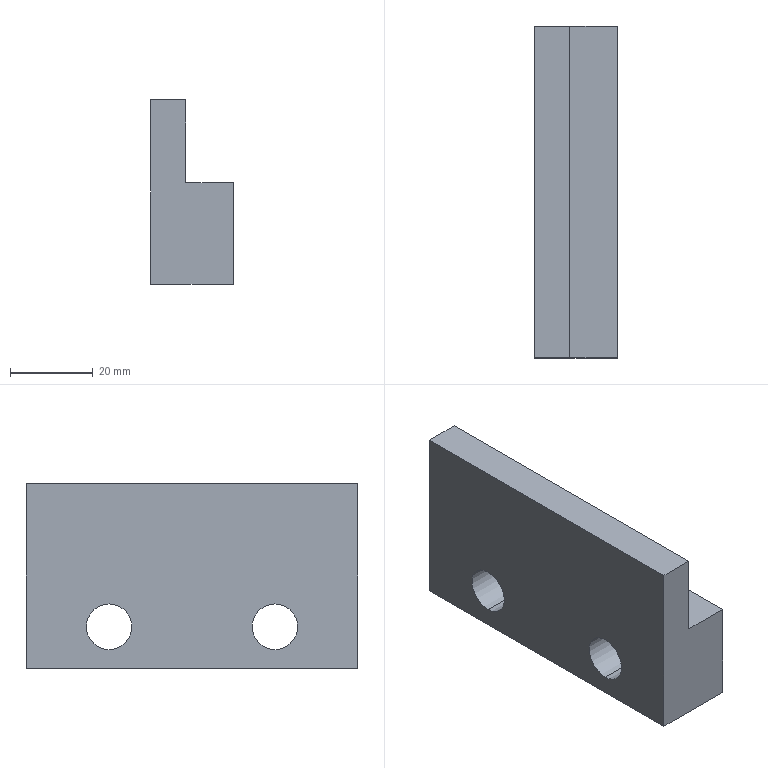Part | SolidWorks | features Extrusion 1, ICE 1 | 1 solid | 12 faces | box 20 x 80 x 44.5 mm | volume 48999 mm3 | plane 8 | cylinder 4 | commonest cylinder face diameters 11 x4
STEP:
#1=CARTESIAN_POINT('',(20.,-20.,-6.75));
#2=VERTEX_POINT('',#1);
#3=CARTESIAN_POINT('',(20.,-20.,-17.75));
#4=VERTEX_POINT('',#3);
#5=CARTESIAN_POINT('',(20.,-20.,-12.25));
#6=DIRECTION('',(1.,0.,0.));
#7=DIRECTION('',(0.,0.,-1.));
#8=AXIS2_PLACEMENT_3D('',#5,#6,#7);
#9=CIRCLE('',#8,5.5);
#10=EDGE_CURVE('',#2,#4,#9,.T.);
#11=ORIENTED_EDGE('',*,*,#10,.T.);
#12=CARTESIAN_POINT('',(0.,-20.,-17.75));
#13=VERTEX_POINT('',#12);
#14=CARTESIAN_POINT('',(20.,-20.,-17.75));
#15=DIRECTION('',(-1.,0.,0.));
#16=VECTOR('',#15,1000.);
#17=LINE('',#14,#16);
#18=EDGE_CURVE('',#4,#13,#17,.T.);
#19=ORIENTED_EDGE('',*,*,#18,.T.);
#20=CARTESIAN_POINT('',(0.,-20.,-6.75));
#21=VERTEX_POINT('',#20);
#22=CARTESIAN_POINT('',(0.,-20.,-12.25));
#23=DIRECTION('',(1.,0.,0.));
#24=DIRECTION('',(0.,0.,-1.));
#25=AXIS2_PLACEMENT_3D('',#22,#23,#24);
#26=CIRCLE('',#25,5.5);
#27=EDGE_CURVE('',#21,#13,#26,.T.);
#28=ORIENTED_EDGE('',*,*,#27,.F.);
#29=CARTESIAN_POINT('',(20.,-20.,-6.75));
#30=DIRECTION('',(-1.,0.,0.));
#31=VECTOR('',#30,1000.);
#32=LINE('',#29,#31);
#33=EDGE_CURVE('',#2,#21,#32,.T.);
#34=ORIENTED_EDGE('',*,*,#33,.F.);
#35=EDGE_LOOP('',(#11,#19,#28,#34));
#36=FACE_OUTER_BOUND('',#35,.T.);
#37=CARTESIAN_POINT('',(20.,-20.,-12.25));
#38=DIRECTION('',(-1.,0.,0.));
#39=DIRECTION('',(0.,0.,1.));
#40=AXIS2_PLACEMENT_3D('',#37,#38,#39);
#41=CYLINDRICAL_SURFACE('',#40,5.5);
#42=ADVANCED_FACE('',(#36),#41,.F.);
#43=CARTESIAN_POINT('',(20.,20.,-6.75));
#44=VERTEX_POINT('',#43);
#45=CARTESIAN_POINT('',(20.,20.,-17.75));
#46=VERTEX_POINT('',#45);
#47=CARTESIAN_POINT('',(20.,20.,-12.25));
#48=DIRECTION('',(1.,0.,0.));
#49=DIRECTION('',(0.,0.,-1.));
#50=AXIS2_PLACEMENT_3D('',#47,#48,#49);
#51=CIRCLE('',#50,5.5);
#52=EDGE_CURVE('',#44,#46,#51,.T.);
#53=ORIENTED_EDGE('',*,*,#52,.T.);
#54=CARTESIAN_POINT('',(0.,20.,-17.75));
#55=VERTEX_POINT('',#54);
#56=CARTESIAN_POINT('',(20.,20.,-17.75));
#57=DIRECTION('',(-1.,0.,0.));
#58=VECTOR('',#57,1000.);
#59=LINE('',#56,#58);
#60=EDGE_CURVE('',#46,#55,#59,.T.);
#61=ORIENTED_EDGE('',*,*,#60,.T.);
#62=CARTESIAN_POINT('',(0.,20.,-6.75));
#63=VERTEX_POINT('',#62);
#64=CARTESIAN_POINT('',(0.,20.,-12.25));
#65=DIRECTION('',(1.,0.,0.));
#66=DIRECTION('',(0.,0.,-1.));
#67=AXIS2_PLACEMENT_3D('',#64,#65,#66);
#68=CIRCLE('',#67,5.5);
#69=EDGE_CURVE('',#63,#55,#68,.T.);
#70=ORIENTED_EDGE('',*,*,#69,.F.);
#71=CARTESIAN_POINT('',(20.,20.,-6.75));
#72=DIRECTION('',(-1.,0.,0.));
#73=VECTOR('',#72,1000.);
#74=LINE('',#71,#73);
#75=EDGE_CURVE('',#44,#63,#74,.T.);
#76=ORIENTED_EDGE('',*,*,#75,.F.);
#77=EDGE_LOOP('',(#53,#61,#70,#76));
#78=FACE_OUTER_BOUND('',#77,.T.);
#79=CARTESIAN_POINT('',(20.,20.,-12.25));
#80=DIRECTION('',(-1.,0.,0.));
#81=DIRECTION('',(0.,0.,1.));
#82=AXIS2_PLACEMENT_3D('',#79,#80,#81);
#83=CYLINDRICAL_SURFACE('',#82,5.5);
#84=ADVANCED_FACE('',(#78),#83,.F.);
#85=CARTESIAN_POINT('',(0.,40.,22.25));
#86=VERTEX_POINT('',#85);
#87=CARTESIAN_POINT('',(0.,40.,-22.25));
#88=VERTEX_POINT('',#87);
#89=CARTESIAN_POINT('',(0.,40.,0.));
#90=DIRECTION('',(0.,0.,-1.));
#91=VECTOR('',#90,1000.);
#92=LINE('',#89,#91);
#93=EDGE_CURVE('',#86,#88,#92,.T.);
#94=ORIENTED_EDGE('',*,*,#93,.F.);
#95=CARTESIAN_POINT('',(8.5,40.,22.25));
#96=VERTEX_POINT('',#95);
#97=CARTESIAN_POINT('',(8.5,40.,22.25));
#98=DIRECTION('',(-1.,0.,0.));
#99=VECTOR('',#98,1000.);
#100=LINE('',#97,#99);
#101=EDGE_CURVE('',#96,#86,#100,.T.);
#102=ORIENTED_EDGE('',*,*,#101,.F.);
#103=CARTESIAN_POINT('',(8.5,40.,2.25));
#104=VERTEX_POINT('',#103);
#105=CARTESIAN_POINT('',(8.5,40.,0.));
#106=DIRECTION('',(0.,0.,-1.));
#107=VECTOR('',#106,1000.);
#108=LINE('',#105,#107);
#109=EDGE_CURVE('',#96,#104,#108,.T.);
#110=ORIENTED_EDGE('',*,*,#109,.T.);
#111=CARTESIAN_POINT('',(20.,40.,2.25));
#112=VERTEX_POINT('',#111);
#113=CARTESIAN_POINT('',(20.,40.,2.25));
#114=DIRECTION('',(-1.,0.,0.));
#115=VECTOR('',#114,1000.);
#116=LINE('',#113,#115);
#117=EDGE_CURVE('',#112,#104,#116,.T.);
#118=ORIENTED_EDGE('',*,*,#117,.F.);
#119=CARTESIAN_POINT('',(20.,40.,-22.25));
#120=VERTEX_POINT('',#119);
#121=CARTESIAN_POINT('',(20.,40.,0.));
#122=DIRECTION('',(0.,0.,-1.));
#123=VECTOR('',#122,1000.);
#124=LINE('',#121,#123);
#125=EDGE_CURVE('',#112,#120,#124,.T.);
#126=ORIENTED_EDGE('',*,*,#125,.T.);
#127=CARTESIAN_POINT('',(20.,40.,-22.25));
#128=DIRECTION('',(-1.,0.,0.));
#129=VECTOR('',#128,1000.);
#130=LINE('',#127,#129);
#131=EDGE_CURVE('',#120,#88,#130,.T.);
#132=ORIENTED_EDGE('',*,*,#131,.T.);
#133=EDGE_LOOP('',(#94,#102,#110,#118,#126,#132));
#134=FACE_OUTER_BOUND('',#133,.T.);
#135=CARTESIAN_POINT('',(8.5,40.,0.));
#136=DIRECTION('',(0.,1.,0.));
#137=DIRECTION('',(0.,0.,1.));
#138=AXIS2_PLACEMENT_3D('',#135,#136,#137);
#139=PLANE('',#138);
#140=ADVANCED_FACE('',(#134),#139,.T.);
#141=CARTESIAN_POINT('',(0.,-40.,22.25));
#142=VERTEX_POINT('',#141);
#143=CARTESIAN_POINT('',(0.,0.,22.25));
#144=DIRECTION('',(0.,1.,0.));
#145=VECTOR('',#144,1000.);
#146=LINE('',#143,#145);
#147=EDGE_CURVE('',#142,#86,#146,.T.);
#148=ORIENTED_EDGE('',*,*,#147,.F.);
#149=CARTESIAN_POINT('',(8.5,-40.,22.25));
#150=VERTEX_POINT('',#149);
#151=CARTESIAN_POINT('',(8.5,-40.,22.25));
#152=DIRECTION('',(-1.,0.,0.));
#153=VECTOR('',#152,1000.);
#154=LINE('',#151,#153);
#155=EDGE_CURVE('',#150,#142,#154,.T.);
#156=ORIENTED_EDGE('',*,*,#155,.F.);
#157=CARTESIAN_POINT('',(8.5,0.,22.25));
#158=DIRECTION('',(0.,1.,0.));
#159=VECTOR('',#158,1000.);
#160=LINE('',#157,#159);
#161=EDGE_CURVE('',#150,#96,#160,.T.);
#162=ORIENTED_EDGE('',*,*,#161,.T.);
#163=ORIENTED_EDGE('',*,*,#101,.T.);
#164=EDGE_LOOP('',(#148,#156,#162,#163));
#165=FACE_OUTER_BOUND('',#164,.T.);
#166=CARTESIAN_POINT('',(8.5,0.,22.25));
#167=DIRECTION('',(0.,0.,1.));
#168=DIRECTION('',(1.,0.,0.));
#169=AXIS2_PLACEMENT_3D('',#166,#167,#168);
#170=PLANE('',#169);
#171=ADVANCED_FACE('',(#165),#170,.T.);
#172=CARTESIAN_POINT('',(0.,-40.,-22.25));
#173=VERTEX_POINT('',#172);
#174=CARTESIAN_POINT('',(0.,-40.,0.));
#175=DIRECTION('',(0.,0.,-1.));
#176=VECTOR('',#175,1000.);
#177=LINE('',#174,#176);
#178=EDGE_CURVE('',#142,#173,#177,.T.);
#179=ORIENTED_EDGE('',*,*,#178,.T.);
#180=CARTESIAN_POINT('',(20.,-40.,-22.25));
#181=VERTEX_POINT('',#180);
#182=CARTESIAN_POINT('',(20.,-40.,-22.25));
#183=DIRECTION('',(-1.,0.,0.));
#184=VECTOR('',#183,1000.);
#185=LINE('',#182,#184);
#186=EDGE_CURVE('',#181,#173,#185,.T.);
#187=ORIENTED_EDGE('',*,*,#186,.F.);
#188=CARTESIAN_POINT('',(20.,-40.,2.25));
#189=VERTEX_POINT('',#188);
#190=CARTESIAN_POINT('',(20.,-40.,0.));
#191=DIRECTION('',(0.,0.,-1.));
#192=VECTOR('',#191,1000.);
#193=LINE('',#190,#192);
#194=EDGE_CURVE('',#189,#181,#193,.T.);
#195=ORIENTED_EDGE('',*,*,#194,.F.);
#196=CARTESIAN_POINT('',(8.5,-40.,2.25));
#197=VERTEX_POINT('',#196);
#198=CARTESIAN_POINT('',(20.,-40.,2.25));
#199=DIRECTION('',(-1.,0.,0.));
#200=VECTOR('',#199,1000.);
#201=LINE('',#198,#200);
#202=EDGE_CURVE('',#189,#197,#201,.T.);
#203=ORIENTED_EDGE('',*,*,#202,.T.);
#204=CARTESIAN_POINT('',(8.5,-40.,0.));
#205=DIRECTION('',(0.,0.,-1.));
#206=VECTOR('',#205,1000.);
#207=LINE('',#204,#206);
#208=EDGE_CURVE('',#150,#197,#207,.T.);
#209=ORIENTED_EDGE('',*,*,#208,.F.);
#210=ORIENTED_EDGE('',*,*,#155,.T.);
#211=EDGE_LOOP('',(#179,#187,#195,#203,#209,#210));
#212=FACE_OUTER_BOUND('',#211,.T.);
#213=CARTESIAN_POINT('',(8.5,-40.,0.));
#214=DIRECTION('',(0.,1.,0.));
#215=DIRECTION('',(0.,0.,1.));
#216=AXIS2_PLACEMENT_3D('',#213,#214,#215);
#217=PLANE('',#216);
#218=ADVANCED_FACE('',(#212),#217,.F.);
#219=CARTESIAN_POINT('',(8.5,0.,2.25));
#220=DIRECTION('',(0.,-1.,0.));
#221=VECTOR('',#220,1000.);
#222=LINE('',#219,#221);
#223=EDGE_CURVE('',#104,#197,#222,.T.);
#224=ORIENTED_EDGE('',*,*,#223,.F.);
#225=ORIENTED_EDGE('',*,*,#109,.F.);
#226=ORIENTED_EDGE('',*,*,#161,.F.);
#227=ORIENTED_EDGE('',*,*,#208,.T.);
#228=EDGE_LOOP('',(#224,#225,#226,#227));
#229=FACE_OUTER_BOUND('',#228,.T.);
#230=CARTESIAN_POINT('',(8.5,0.,0.));
#231=DIRECTION('',(1.,0.,0.));
#232=DIRECTION('',(0.,0.,-1.));
#233=AXIS2_PLACEMENT_3D('',#230,#231,#232);
#234=PLANE('',#233);
#235=ADVANCED_FACE('',(#229),#234,.T.);
#236=ORIENTED_EDGE('',*,*,#93,.T.);
#237=CARTESIAN_POINT('',(0.,0.,-22.25));
#238=DIRECTION('',(0.,1.,0.));
#239=VECTOR('',#238,1000.);
#240=LINE('',#237,#239);
#241=EDGE_CURVE('',#173,#88,#240,.T.);
#242=ORIENTED_EDGE('',*,*,#241,.F.);
#243=ORIENTED_EDGE('',*,*,#178,.F.);
#244=ORIENTED_EDGE('',*,*,#147,.T.);
#245=EDGE_LOOP('',(#236,#242,#243,#244));
#246=FACE_OUTER_BOUND('',#245,.T.);
#247=ORIENTED_EDGE('',*,*,#27,.T.);
#248=CARTESIAN_POINT('',(0.,-20.,-12.25));
#249=DIRECTION('',(1.,0.,0.));
#250=DIRECTION('',(0.,0.,-1.));
#251=AXIS2_PLACEMENT_3D('',#248,#249,#250);
#252=CIRCLE('',#251,5.5);
#253=EDGE_CURVE('',#13,#21,#252,.T.);
#254=ORIENTED_EDGE('',*,*,#253,.T.);
#255=EDGE_LOOP('',(#247,#254));
#256=FACE_BOUND('',#255,.T.);
#257=ORIENTED_EDGE('',*,*,#69,.T.);
#258=CARTESIAN_POINT('',(0.,20.,-12.25));
#259=DIRECTION('',(1.,0.,0.));
#260=DIRECTION('',(0.,0.,-1.));
#261=AXIS2_PLACEMENT_3D('',#258,#259,#260);
#262=CIRCLE('',#261,5.5);
#263=EDGE_CURVE('',#55,#63,#262,.T.);
#264=ORIENTED_EDGE('',*,*,#263,.T.);
#265=EDGE_LOOP('',(#257,#264));
#266=FACE_BOUND('',#265,.T.);
#267=CARTESIAN_POINT('',(0.,0.,0.));
#268=DIRECTION('',(1.,0.,0.));
#269=DIRECTION('',(0.,0.,-1.));
#270=AXIS2_PLACEMENT_3D('',#267,#268,#269);
#271=PLANE('',#270);
#272=ADVANCED_FACE('',(#246,#256,#266),#271,.F.);
#273=ORIENTED_EDGE('',*,*,#117,.T.);
#274=ORIENTED_EDGE('',*,*,#223,.T.);
#275=ORIENTED_EDGE('',*,*,#202,.F.);
#276=CARTESIAN_POINT('',(20.,0.,2.25));
#277=DIRECTION('',(0.,-1.,0.));
#278=VECTOR('',#277,1000.);
#279=LINE('',#276,#278);
#280=EDGE_CURVE('',#112,#189,#279,.T.);
#281=ORIENTED_EDGE('',*,*,#280,.F.);
#282=EDGE_LOOP('',(#273,#274,#275,#281));
#283=FACE_OUTER_BOUND('',#282,.T.);
#284=CARTESIAN_POINT('',(20.,0.,2.25));
#285=DIRECTION('',(0.,0.,-1.));
#286=DIRECTION('',(0.,1.,0.));
#287=AXIS2_PLACEMENT_3D('',#284,#285,#286);
#288=PLANE('',#287);
#289=ADVANCED_FACE('',(#283),#288,.F.);
#290=ORIENTED_EDGE('',*,*,#60,.F.);
#291=CARTESIAN_POINT('',(20.,20.,-12.25));
#292=DIRECTION('',(1.,0.,0.));
#293=DIRECTION('',(0.,0.,-1.));
#294=AXIS2_PLACEMENT_3D('',#291,#292,#293);
#295=CIRCLE('',#294,5.5);
#296=EDGE_CURVE('',#46,#44,#295,.T.);
#297=ORIENTED_EDGE('',*,*,#296,.T.);
#298=ORIENTED_EDGE('',*,*,#75,.T.);
#299=ORIENTED_EDGE('',*,*,#263,.F.);
#300=EDGE_LOOP('',(#290,#297,#298,#299));
#301=FACE_OUTER_BOUND('',#300,.T.);
#302=CARTESIAN_POINT('',(20.,20.,-12.25));
#303=DIRECTION('',(-1.,0.,0.));
#304=DIRECTION('',(0.,0.,1.));
#305=AXIS2_PLACEMENT_3D('',#302,#303,#304);
#306=CYLINDRICAL_SURFACE('',#305,5.5);
#307=ADVANCED_FACE('',(#301),#306,.F.);
#308=ORIENTED_EDGE('',*,*,#18,.F.);
#309=CARTESIAN_POINT('',(20.,-20.,-12.25));
#310=DIRECTION('',(1.,0.,0.));
#311=DIRECTION('',(0.,0.,-1.));
#312=AXIS2_PLACEMENT_3D('',#309,#310,#311);
#313=CIRCLE('',#312,5.5);
#314=EDGE_CURVE('',#4,#2,#313,.T.);
#315=ORIENTED_EDGE('',*,*,#314,.T.);
#316=ORIENTED_EDGE('',*,*,#33,.T.);
#317=ORIENTED_EDGE('',*,*,#253,.F.);
#318=EDGE_LOOP('',(#308,#315,#316,#317));
#319=FACE_OUTER_BOUND('',#318,.T.);
#320=CARTESIAN_POINT('',(20.,-20.,-12.25));
#321=DIRECTION('',(-1.,0.,0.));
#322=DIRECTION('',(0.,0.,1.));
#323=AXIS2_PLACEMENT_3D('',#320,#321,#322);
#324=CYLINDRICAL_SURFACE('',#323,5.5);
#325=ADVANCED_FACE('',(#319),#324,.F.);
#326=ORIENTED_EDGE('',*,*,#241,.T.);
#327=ORIENTED_EDGE('',*,*,#131,.F.);
#328=CARTESIAN_POINT('',(20.,0.,-22.25));
#329=DIRECTION('',(0.,1.,0.));
#330=VECTOR('',#329,1000.);
#331=LINE('',#328,#330);
#332=EDGE_CURVE('',#181,#120,#331,.T.);
#333=ORIENTED_EDGE('',*,*,#332,.F.);
#334=ORIENTED_EDGE('',*,*,#186,.T.);
#335=EDGE_LOOP('',(#326,#327,#333,#334));
#336=FACE_OUTER_BOUND('',#335,.T.);
#337=CARTESIAN_POINT('',(20.,0.,-22.25));
#338=DIRECTION('',(0.,0.,1.));
#339=DIRECTION('',(1.,0.,0.));
#340=AXIS2_PLACEMENT_3D('',#337,#338,#339);
#341=PLANE('',#340);
#342=ADVANCED_FACE('',(#336),#341,.F.);
#343=ORIENTED_EDGE('',*,*,#10,.F.);
#344=ORIENTED_EDGE('',*,*,#314,.F.);
#345=EDGE_LOOP('',(#343,#344));
#346=FACE_BOUND('',#345,.T.);
#347=ORIENTED_EDGE('',*,*,#52,.F.);
#348=ORIENTED_EDGE('',*,*,#296,.F.);
#349=EDGE_LOOP('',(#347,#348));
#350=FACE_BOUND('',#349,.T.);
#351=ORIENTED_EDGE('',*,*,#125,.F.);
#352=ORIENTED_EDGE('',*,*,#280,.T.);
#353=ORIENTED_EDGE('',*,*,#194,.T.);
#354=ORIENTED_EDGE('',*,*,#332,.T.);
#355=EDGE_LOOP('',(#351,#352,#353,#354));
#356=FACE_OUTER_BOUND('',#355,.T.);
#357=CARTESIAN_POINT('',(20.,0.,0.));
#358=DIRECTION('',(1.,0.,0.));
#359=DIRECTION('',(0.,0.,-1.));
#360=AXIS2_PLACEMENT_3D('',#357,#358,#359);
#361=PLANE('',#360);
#362=ADVANCED_FACE('',(#346,#350,#356),#361,.T.);
#363=CLOSED_SHELL('',(#42,#84,#140,#171,#218,#235,#272,#289,#307,#325,#342,#362));
#364=MANIFOLD_SOLID_BREP('',#363);
#365=CARTESIAN_POINT('',(0.,0.,0.));
#366=DIRECTION('',(0.,0.,1.));
#367=DIRECTION('',(1.,0.,0.));
#368=AXIS2_PLACEMENT_3D('',#365,#366,#367);
#369=(LENGTH_UNIT()NAMED_UNIT(*)SI_UNIT(.MILLI.,.METRE.));
#370=UNCERTAINTY_MEASURE_WITH_UNIT(LENGTH_MEASURE(0.00001),#369,'','');
#371=(NAMED_UNIT(*)PLANE_ANGLE_UNIT()SI_UNIT($,.RADIAN.));
#372=(NAMED_UNIT(*)SI_UNIT($,.STERADIAN.)SOLID_ANGLE_UNIT());
#373=(GEOMETRIC_REPRESENTATION_CONTEXT(3)GLOBAL_UNCERTAINTY_ASSIGNED_CONTEXT((#370))GLOBAL_UNIT_ASSIGNED_CONTEXT((#369,#371,#372))REPRESENTATION_CONTEXT('',''));
#374=ADVANCED_BREP_SHAPE_REPRESENTATION('',(#364,#368),#373);